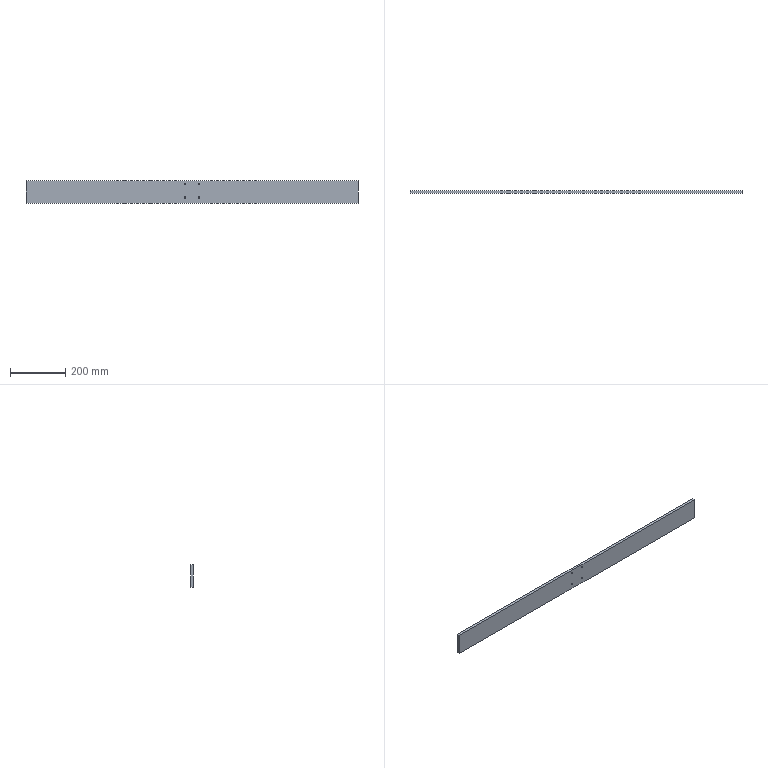Part | SolidWorks | features Extrusion 1, ICE 1 | 1 solid | 14 faces | box 1200 x 10 x 80 mm | volume 959446 mm3 | cylinder 8 | plane 6 | commonest cylinder face diameters 4.2 x8
STEP:
#1=CARTESIAN_POINT('',(-25.,-5.,-22.1));
#2=VERTEX_POINT('',#1);
#3=CARTESIAN_POINT('',(-25.,-5.,-17.9));
#4=VERTEX_POINT('',#3);
#5=CARTESIAN_POINT('',(-25.,-5.,-20.));
#6=DIRECTION('',(0.,1.,0.));
#7=DIRECTION('',(0.,0.,1.));
#8=AXIS2_PLACEMENT_3D('',#5,#6,#7);
#9=CIRCLE('',#8,2.1);
#10=EDGE_CURVE('',#2,#4,#9,.T.);
#11=ORIENTED_EDGE('',*,*,#10,.F.);
#12=CARTESIAN_POINT('',(-25.,5.,-22.1));
#13=VERTEX_POINT('',#12);
#14=CARTESIAN_POINT('',(-25.,-21.,-22.1));
#15=DIRECTION('',(0.,1.,0.));
#16=VECTOR('',#15,1000.);
#17=LINE('',#14,#16);
#18=EDGE_CURVE('',#2,#13,#17,.T.);
#19=ORIENTED_EDGE('',*,*,#18,.T.);
#20=CARTESIAN_POINT('',(-25.,5.,-17.9));
#21=VERTEX_POINT('',#20);
#22=CARTESIAN_POINT('',(-25.,5.,-20.));
#23=DIRECTION('',(0.,1.,0.));
#24=DIRECTION('',(0.,0.,1.));
#25=AXIS2_PLACEMENT_3D('',#22,#23,#24);
#26=CIRCLE('',#25,2.1);
#27=EDGE_CURVE('',#13,#21,#26,.T.);
#28=ORIENTED_EDGE('',*,*,#27,.T.);
#29=CARTESIAN_POINT('',(-25.,-21.,-17.9));
#30=DIRECTION('',(0.,1.,0.));
#31=VECTOR('',#30,1000.);
#32=LINE('',#29,#31);
#33=EDGE_CURVE('',#4,#21,#32,.T.);
#34=ORIENTED_EDGE('',*,*,#33,.F.);
#35=EDGE_LOOP('',(#11,#19,#28,#34));
#36=FACE_OUTER_BOUND('',#35,.T.);
#37=CARTESIAN_POINT('',(-25.,-21.,-20.));
#38=DIRECTION('',(0.,1.,0.));
#39=DIRECTION('',(0.,0.,1.));
#40=AXIS2_PLACEMENT_3D('',#37,#38,#39);
#41=CYLINDRICAL_SURFACE('',#40,2.1);
#42=ADVANCED_FACE('',(#36),#41,.F.);
#43=CARTESIAN_POINT('',(25.,-5.,27.9));
#44=VERTEX_POINT('',#43);
#45=CARTESIAN_POINT('',(25.,-5.,32.1));
#46=VERTEX_POINT('',#45);
#47=CARTESIAN_POINT('',(25.,-5.,30.));
#48=DIRECTION('',(0.,1.,0.));
#49=DIRECTION('',(0.,0.,1.));
#50=AXIS2_PLACEMENT_3D('',#47,#48,#49);
#51=CIRCLE('',#50,2.1);
#52=EDGE_CURVE('',#44,#46,#51,.T.);
#53=ORIENTED_EDGE('',*,*,#52,.F.);
#54=CARTESIAN_POINT('',(25.,5.,27.9));
#55=VERTEX_POINT('',#54);
#56=CARTESIAN_POINT('',(25.,-21.,27.9));
#57=DIRECTION('',(0.,1.,0.));
#58=VECTOR('',#57,1000.);
#59=LINE('',#56,#58);
#60=EDGE_CURVE('',#44,#55,#59,.T.);
#61=ORIENTED_EDGE('',*,*,#60,.T.);
#62=CARTESIAN_POINT('',(25.,5.,32.1));
#63=VERTEX_POINT('',#62);
#64=CARTESIAN_POINT('',(25.,5.,30.));
#65=DIRECTION('',(0.,1.,0.));
#66=DIRECTION('',(0.,0.,1.));
#67=AXIS2_PLACEMENT_3D('',#64,#65,#66);
#68=CIRCLE('',#67,2.1);
#69=EDGE_CURVE('',#55,#63,#68,.T.);
#70=ORIENTED_EDGE('',*,*,#69,.T.);
#71=CARTESIAN_POINT('',(25.,-21.,32.1));
#72=DIRECTION('',(0.,1.,0.));
#73=VECTOR('',#72,1000.);
#74=LINE('',#71,#73);
#75=EDGE_CURVE('',#46,#63,#74,.T.);
#76=ORIENTED_EDGE('',*,*,#75,.F.);
#77=EDGE_LOOP('',(#53,#61,#70,#76));
#78=FACE_OUTER_BOUND('',#77,.T.);
#79=CARTESIAN_POINT('',(25.,-21.,30.));
#80=DIRECTION('',(0.,1.,0.));
#81=DIRECTION('',(0.,0.,1.));
#82=AXIS2_PLACEMENT_3D('',#79,#80,#81);
#83=CYLINDRICAL_SURFACE('',#82,2.1);
#84=ADVANCED_FACE('',(#78),#83,.F.);
#85=CARTESIAN_POINT('',(-25.,-5.,27.9));
#86=VERTEX_POINT('',#85);
#87=CARTESIAN_POINT('',(-25.,-5.,32.1));
#88=VERTEX_POINT('',#87);
#89=CARTESIAN_POINT('',(-25.,-5.,30.));
#90=DIRECTION('',(0.,1.,0.));
#91=DIRECTION('',(0.,0.,1.));
#92=AXIS2_PLACEMENT_3D('',#89,#90,#91);
#93=CIRCLE('',#92,2.1);
#94=EDGE_CURVE('',#86,#88,#93,.T.);
#95=ORIENTED_EDGE('',*,*,#94,.F.);
#96=CARTESIAN_POINT('',(-25.,5.,27.9));
#97=VERTEX_POINT('',#96);
#98=CARTESIAN_POINT('',(-25.,-21.,27.9));
#99=DIRECTION('',(0.,1.,0.));
#100=VECTOR('',#99,1000.);
#101=LINE('',#98,#100);
#102=EDGE_CURVE('',#86,#97,#101,.T.);
#103=ORIENTED_EDGE('',*,*,#102,.T.);
#104=CARTESIAN_POINT('',(-25.,5.,32.1));
#105=VERTEX_POINT('',#104);
#106=CARTESIAN_POINT('',(-25.,5.,30.));
#107=DIRECTION('',(0.,1.,0.));
#108=DIRECTION('',(0.,0.,1.));
#109=AXIS2_PLACEMENT_3D('',#106,#107,#108);
#110=CIRCLE('',#109,2.1);
#111=EDGE_CURVE('',#97,#105,#110,.T.);
#112=ORIENTED_EDGE('',*,*,#111,.T.);
#113=CARTESIAN_POINT('',(-25.,-21.,32.1));
#114=DIRECTION('',(0.,1.,0.));
#115=VECTOR('',#114,1000.);
#116=LINE('',#113,#115);
#117=EDGE_CURVE('',#88,#105,#116,.T.);
#118=ORIENTED_EDGE('',*,*,#117,.F.);
#119=EDGE_LOOP('',(#95,#103,#112,#118));
#120=FACE_OUTER_BOUND('',#119,.T.);
#121=CARTESIAN_POINT('',(-25.,-21.,30.));
#122=DIRECTION('',(0.,1.,0.));
#123=DIRECTION('',(0.,0.,1.));
#124=AXIS2_PLACEMENT_3D('',#121,#122,#123);
#125=CYLINDRICAL_SURFACE('',#124,2.1);
#126=ADVANCED_FACE('',(#120),#125,.F.);
#127=CARTESIAN_POINT('',(25.,-5.,-22.1));
#128=VERTEX_POINT('',#127);
#129=CARTESIAN_POINT('',(25.,-5.,-17.9));
#130=VERTEX_POINT('',#129);
#131=CARTESIAN_POINT('',(25.,-5.,-20.));
#132=DIRECTION('',(0.,1.,0.));
#133=DIRECTION('',(0.,0.,1.));
#134=AXIS2_PLACEMENT_3D('',#131,#132,#133);
#135=CIRCLE('',#134,2.1);
#136=EDGE_CURVE('',#128,#130,#135,.T.);
#137=ORIENTED_EDGE('',*,*,#136,.F.);
#138=CARTESIAN_POINT('',(25.,5.,-22.1));
#139=VERTEX_POINT('',#138);
#140=CARTESIAN_POINT('',(25.,-21.,-22.1));
#141=DIRECTION('',(0.,1.,0.));
#142=VECTOR('',#141,1000.);
#143=LINE('',#140,#142);
#144=EDGE_CURVE('',#128,#139,#143,.T.);
#145=ORIENTED_EDGE('',*,*,#144,.T.);
#146=CARTESIAN_POINT('',(25.,5.,-17.9));
#147=VERTEX_POINT('',#146);
#148=CARTESIAN_POINT('',(25.,5.,-20.));
#149=DIRECTION('',(0.,1.,0.));
#150=DIRECTION('',(0.,0.,1.));
#151=AXIS2_PLACEMENT_3D('',#148,#149,#150);
#152=CIRCLE('',#151,2.1);
#153=EDGE_CURVE('',#139,#147,#152,.T.);
#154=ORIENTED_EDGE('',*,*,#153,.T.);
#155=CARTESIAN_POINT('',(25.,-21.,-17.9));
#156=DIRECTION('',(0.,1.,0.));
#157=VECTOR('',#156,1000.);
#158=LINE('',#155,#157);
#159=EDGE_CURVE('',#130,#147,#158,.T.);
#160=ORIENTED_EDGE('',*,*,#159,.F.);
#161=EDGE_LOOP('',(#137,#145,#154,#160));
#162=FACE_OUTER_BOUND('',#161,.T.);
#163=CARTESIAN_POINT('',(25.,-21.,-20.));
#164=DIRECTION('',(0.,1.,0.));
#165=DIRECTION('',(0.,0.,1.));
#166=AXIS2_PLACEMENT_3D('',#163,#164,#165);
#167=CYLINDRICAL_SURFACE('',#166,2.1);
#168=ADVANCED_FACE('',(#162),#167,.F.);
#169=CARTESIAN_POINT('',(600.,-5.,40.));
#170=VERTEX_POINT('',#169);
#171=CARTESIAN_POINT('',(600.,-5.,-40.));
#172=VERTEX_POINT('',#171);
#173=CARTESIAN_POINT('',(600.,-5.,-40.));
#174=DIRECTION('',(0.,0.,-1.));
#175=VECTOR('',#174,1000.);
#176=LINE('',#173,#175);
#177=EDGE_CURVE('',#170,#172,#176,.T.);
#178=ORIENTED_EDGE('',*,*,#177,.T.);
#179=CARTESIAN_POINT('',(600.,5.,-40.));
#180=VERTEX_POINT('',#179);
#181=CARTESIAN_POINT('',(600.,5.,-40.));
#182=DIRECTION('',(0.,-1.,0.));
#183=VECTOR('',#182,1000.);
#184=LINE('',#181,#183);
#185=EDGE_CURVE('',#180,#172,#184,.T.);
#186=ORIENTED_EDGE('',*,*,#185,.F.);
#187=CARTESIAN_POINT('',(600.,5.,40.));
#188=VERTEX_POINT('',#187);
#189=CARTESIAN_POINT('',(600.,5.,-40.));
#190=DIRECTION('',(0.,0.,-1.));
#191=VECTOR('',#190,1000.);
#192=LINE('',#189,#191);
#193=EDGE_CURVE('',#188,#180,#192,.T.);
#194=ORIENTED_EDGE('',*,*,#193,.F.);
#195=CARTESIAN_POINT('',(600.,5.,40.));
#196=DIRECTION('',(0.,-1.,0.));
#197=VECTOR('',#196,1000.);
#198=LINE('',#195,#197);
#199=EDGE_CURVE('',#188,#170,#198,.T.);
#200=ORIENTED_EDGE('',*,*,#199,.T.);
#201=EDGE_LOOP('',(#178,#186,#194,#200));
#202=FACE_OUTER_BOUND('',#201,.T.);
#203=CARTESIAN_POINT('',(600.,5.,-40.));
#204=DIRECTION('',(-1.,0.,0.));
#205=DIRECTION('',(0.,0.,1.));
#206=AXIS2_PLACEMENT_3D('',#203,#204,#205);
#207=PLANE('',#206);
#208=ADVANCED_FACE('',(#202),#207,.F.);
#209=CARTESIAN_POINT('',(-600.,-5.,-40.));
#210=VERTEX_POINT('',#209);
#211=CARTESIAN_POINT('',(-600.,-5.,-40.));
#212=DIRECTION('',(-1.,0.,0.));
#213=VECTOR('',#212,1000.);
#214=LINE('',#211,#213);
#215=EDGE_CURVE('',#172,#210,#214,.T.);
#216=ORIENTED_EDGE('',*,*,#215,.T.);
#217=CARTESIAN_POINT('',(-600.,5.,-40.));
#218=VERTEX_POINT('',#217);
#219=CARTESIAN_POINT('',(-600.,5.,-40.));
#220=DIRECTION('',(0.,-1.,0.));
#221=VECTOR('',#220,1000.);
#222=LINE('',#219,#221);
#223=EDGE_CURVE('',#218,#210,#222,.T.);
#224=ORIENTED_EDGE('',*,*,#223,.F.);
#225=CARTESIAN_POINT('',(-600.,5.,-40.));
#226=DIRECTION('',(-1.,0.,0.));
#227=VECTOR('',#226,1000.);
#228=LINE('',#225,#227);
#229=EDGE_CURVE('',#180,#218,#228,.T.);
#230=ORIENTED_EDGE('',*,*,#229,.F.);
#231=ORIENTED_EDGE('',*,*,#185,.T.);
#232=EDGE_LOOP('',(#216,#224,#230,#231));
#233=FACE_OUTER_BOUND('',#232,.T.);
#234=CARTESIAN_POINT('',(-600.,5.,-40.));
#235=DIRECTION('',(0.,0.,1.));
#236=DIRECTION('',(1.,0.,0.));
#237=AXIS2_PLACEMENT_3D('',#234,#235,#236);
#238=PLANE('',#237);
#239=ADVANCED_FACE('',(#233),#238,.F.);
#240=CARTESIAN_POINT('',(-600.,-5.,40.));
#241=VERTEX_POINT('',#240);
#242=CARTESIAN_POINT('',(-600.,-5.,-40.));
#243=DIRECTION('',(0.,0.,1.));
#244=VECTOR('',#243,1000.);
#245=LINE('',#242,#244);
#246=EDGE_CURVE('',#210,#241,#245,.T.);
#247=ORIENTED_EDGE('',*,*,#246,.T.);
#248=CARTESIAN_POINT('',(-600.,5.,40.));
#249=VERTEX_POINT('',#248);
#250=CARTESIAN_POINT('',(-600.,5.,40.));
#251=DIRECTION('',(0.,-1.,0.));
#252=VECTOR('',#251,1000.);
#253=LINE('',#250,#252);
#254=EDGE_CURVE('',#249,#241,#253,.T.);
#255=ORIENTED_EDGE('',*,*,#254,.F.);
#256=CARTESIAN_POINT('',(-600.,5.,-40.));
#257=DIRECTION('',(0.,0.,1.));
#258=VECTOR('',#257,1000.);
#259=LINE('',#256,#258);
#260=EDGE_CURVE('',#218,#249,#259,.T.);
#261=ORIENTED_EDGE('',*,*,#260,.F.);
#262=ORIENTED_EDGE('',*,*,#223,.T.);
#263=EDGE_LOOP('',(#247,#255,#261,#262));
#264=FACE_OUTER_BOUND('',#263,.T.);
#265=CARTESIAN_POINT('',(-600.,5.,-40.));
#266=DIRECTION('',(1.,0.,0.));
#267=DIRECTION('',(0.,0.,-1.));
#268=AXIS2_PLACEMENT_3D('',#265,#266,#267);
#269=PLANE('',#268);
#270=ADVANCED_FACE('',(#264),#269,.F.);
#271=CARTESIAN_POINT('',(-600.,-5.,40.));
#272=DIRECTION('',(1.,0.,0.));
#273=VECTOR('',#272,1000.);
#274=LINE('',#271,#273);
#275=EDGE_CURVE('',#241,#170,#274,.T.);
#276=ORIENTED_EDGE('',*,*,#275,.T.);
#277=ORIENTED_EDGE('',*,*,#199,.F.);
#278=CARTESIAN_POINT('',(-600.,5.,40.));
#279=DIRECTION('',(1.,0.,0.));
#280=VECTOR('',#279,1000.);
#281=LINE('',#278,#280);
#282=EDGE_CURVE('',#249,#188,#281,.T.);
#283=ORIENTED_EDGE('',*,*,#282,.F.);
#284=ORIENTED_EDGE('',*,*,#254,.T.);
#285=EDGE_LOOP('',(#276,#277,#283,#284));
#286=FACE_OUTER_BOUND('',#285,.T.);
#287=CARTESIAN_POINT('',(-600.,5.,40.));
#288=DIRECTION('',(0.,0.,-1.));
#289=DIRECTION('',(-1.,0.,0.));
#290=AXIS2_PLACEMENT_3D('',#287,#288,#289);
#291=PLANE('',#290);
#292=ADVANCED_FACE('',(#286),#291,.F.);
#293=CARTESIAN_POINT('',(-25.,5.,-20.));
#294=DIRECTION('',(0.,1.,0.));
#295=DIRECTION('',(0.,0.,1.));
#296=AXIS2_PLACEMENT_3D('',#293,#294,#295);
#297=CIRCLE('',#296,2.1);
#298=EDGE_CURVE('',#21,#13,#297,.T.);
#299=ORIENTED_EDGE('',*,*,#298,.F.);
#300=ORIENTED_EDGE('',*,*,#27,.F.);
#301=EDGE_LOOP('',(#299,#300));
#302=FACE_BOUND('',#301,.T.);
#303=CARTESIAN_POINT('',(25.,5.,30.));
#304=DIRECTION('',(0.,1.,0.));
#305=DIRECTION('',(0.,0.,1.));
#306=AXIS2_PLACEMENT_3D('',#303,#304,#305);
#307=CIRCLE('',#306,2.1);
#308=EDGE_CURVE('',#63,#55,#307,.T.);
#309=ORIENTED_EDGE('',*,*,#308,.F.);
#310=ORIENTED_EDGE('',*,*,#69,.F.);
#311=EDGE_LOOP('',(#309,#310));
#312=FACE_BOUND('',#311,.T.);
#313=CARTESIAN_POINT('',(-25.,5.,30.));
#314=DIRECTION('',(0.,1.,0.));
#315=DIRECTION('',(0.,0.,1.));
#316=AXIS2_PLACEMENT_3D('',#313,#314,#315);
#317=CIRCLE('',#316,2.1);
#318=EDGE_CURVE('',#105,#97,#317,.T.);
#319=ORIENTED_EDGE('',*,*,#318,.F.);
#320=ORIENTED_EDGE('',*,*,#111,.F.);
#321=EDGE_LOOP('',(#319,#320));
#322=FACE_BOUND('',#321,.T.);
#323=CARTESIAN_POINT('',(25.,5.,-20.));
#324=DIRECTION('',(0.,1.,0.));
#325=DIRECTION('',(0.,0.,1.));
#326=AXIS2_PLACEMENT_3D('',#323,#324,#325);
#327=CIRCLE('',#326,2.1);
#328=EDGE_CURVE('',#147,#139,#327,.T.);
#329=ORIENTED_EDGE('',*,*,#328,.F.);
#330=ORIENTED_EDGE('',*,*,#153,.F.);
#331=EDGE_LOOP('',(#329,#330));
#332=FACE_BOUND('',#331,.T.);
#333=ORIENTED_EDGE('',*,*,#193,.T.);
#334=ORIENTED_EDGE('',*,*,#229,.T.);
#335=ORIENTED_EDGE('',*,*,#260,.T.);
#336=ORIENTED_EDGE('',*,*,#282,.T.);
#337=EDGE_LOOP('',(#333,#334,#335,#336));
#338=FACE_OUTER_BOUND('',#337,.T.);
#339=CARTESIAN_POINT('',(0.,5.,0.));
#340=DIRECTION('',(0.,1.,0.));
#341=DIRECTION('',(0.,0.,1.));
#342=AXIS2_PLACEMENT_3D('',#339,#340,#341);
#343=PLANE('',#342);
#344=ADVANCED_FACE('',(#302,#312,#322,#332,#338),#343,.T.);
#345=CARTESIAN_POINT('',(-25.,-5.,-20.));
#346=DIRECTION('',(0.,1.,0.));
#347=DIRECTION('',(0.,0.,1.));
#348=AXIS2_PLACEMENT_3D('',#345,#346,#347);
#349=CIRCLE('',#348,2.1);
#350=EDGE_CURVE('',#4,#2,#349,.T.);
#351=ORIENTED_EDGE('',*,*,#350,.T.);
#352=ORIENTED_EDGE('',*,*,#10,.T.);
#353=EDGE_LOOP('',(#351,#352));
#354=FACE_BOUND('',#353,.T.);
#355=CARTESIAN_POINT('',(25.,-5.,30.));
#356=DIRECTION('',(0.,1.,0.));
#357=DIRECTION('',(0.,0.,1.));
#358=AXIS2_PLACEMENT_3D('',#355,#356,#357);
#359=CIRCLE('',#358,2.1);
#360=EDGE_CURVE('',#46,#44,#359,.T.);
#361=ORIENTED_EDGE('',*,*,#360,.T.);
#362=ORIENTED_EDGE('',*,*,#52,.T.);
#363=EDGE_LOOP('',(#361,#362));
#364=FACE_BOUND('',#363,.T.);
#365=CARTESIAN_POINT('',(-25.,-5.,30.));
#366=DIRECTION('',(0.,1.,0.));
#367=DIRECTION('',(0.,0.,1.));
#368=AXIS2_PLACEMENT_3D('',#365,#366,#367);
#369=CIRCLE('',#368,2.1);
#370=EDGE_CURVE('',#88,#86,#369,.T.);
#371=ORIENTED_EDGE('',*,*,#370,.T.);
#372=ORIENTED_EDGE('',*,*,#94,.T.);
#373=EDGE_LOOP('',(#371,#372));
#374=FACE_BOUND('',#373,.T.);
#375=CARTESIAN_POINT('',(25.,-5.,-20.));
#376=DIRECTION('',(0.,1.,0.));
#377=DIRECTION('',(0.,0.,1.));
#378=AXIS2_PLACEMENT_3D('',#375,#376,#377);
#379=CIRCLE('',#378,2.1);
#380=EDGE_CURVE('',#130,#128,#379,.T.);
#381=ORIENTED_EDGE('',*,*,#380,.T.);
#382=ORIENTED_EDGE('',*,*,#136,.T.);
#383=EDGE_LOOP('',(#381,#382));
#384=FACE_BOUND('',#383,.T.);
#385=ORIENTED_EDGE('',*,*,#177,.F.);
#386=ORIENTED_EDGE('',*,*,#275,.F.);
#387=ORIENTED_EDGE('',*,*,#246,.F.);
#388=ORIENTED_EDGE('',*,*,#215,.F.);
#389=EDGE_LOOP('',(#385,#386,#387,#388));
#390=FACE_OUTER_BOUND('',#389,.T.);
#391=CARTESIAN_POINT('',(0.,-5.,0.));
#392=DIRECTION('',(0.,1.,0.));
#393=DIRECTION('',(0.,0.,1.));
#394=AXIS2_PLACEMENT_3D('',#391,#392,#393);
#395=PLANE('',#394);
#396=ADVANCED_FACE('',(#354,#364,#374,#384,#390),#395,.F.);
#397=ORIENTED_EDGE('',*,*,#144,.F.);
#398=ORIENTED_EDGE('',*,*,#380,.F.);
#399=ORIENTED_EDGE('',*,*,#159,.T.);
#400=ORIENTED_EDGE('',*,*,#328,.T.);
#401=EDGE_LOOP('',(#397,#398,#399,#400));
#402=FACE_OUTER_BOUND('',#401,.T.);
#403=CARTESIAN_POINT('',(25.,-21.,-20.));
#404=DIRECTION('',(0.,1.,0.));
#405=DIRECTION('',(0.,0.,1.));
#406=AXIS2_PLACEMENT_3D('',#403,#404,#405);
#407=CYLINDRICAL_SURFACE('',#406,2.1);
#408=ADVANCED_FACE('',(#402),#407,.F.);
#409=ORIENTED_EDGE('',*,*,#102,.F.);
#410=ORIENTED_EDGE('',*,*,#370,.F.);
#411=ORIENTED_EDGE('',*,*,#117,.T.);
#412=ORIENTED_EDGE('',*,*,#318,.T.);
#413=EDGE_LOOP('',(#409,#410,#411,#412));
#414=FACE_OUTER_BOUND('',#413,.T.);
#415=CARTESIAN_POINT('',(-25.,-21.,30.));
#416=DIRECTION('',(0.,1.,0.));
#417=DIRECTION('',(0.,0.,1.));
#418=AXIS2_PLACEMENT_3D('',#415,#416,#417);
#419=CYLINDRICAL_SURFACE('',#418,2.1);
#420=ADVANCED_FACE('',(#414),#419,.F.);
#421=ORIENTED_EDGE('',*,*,#60,.F.);
#422=ORIENTED_EDGE('',*,*,#360,.F.);
#423=ORIENTED_EDGE('',*,*,#75,.T.);
#424=ORIENTED_EDGE('',*,*,#308,.T.);
#425=EDGE_LOOP('',(#421,#422,#423,#424));
#426=FACE_OUTER_BOUND('',#425,.T.);
#427=CARTESIAN_POINT('',(25.,-21.,30.));
#428=DIRECTION('',(0.,1.,0.));
#429=DIRECTION('',(0.,0.,1.));
#430=AXIS2_PLACEMENT_3D('',#427,#428,#429);
#431=CYLINDRICAL_SURFACE('',#430,2.1);
#432=ADVANCED_FACE('',(#426),#431,.F.);
#433=ORIENTED_EDGE('',*,*,#18,.F.);
#434=ORIENTED_EDGE('',*,*,#350,.F.);
#435=ORIENTED_EDGE('',*,*,#33,.T.);
#436=ORIENTED_EDGE('',*,*,#298,.T.);
#437=EDGE_LOOP('',(#433,#434,#435,#436));
#438=FACE_OUTER_BOUND('',#437,.T.);
#439=CARTESIAN_POINT('',(-25.,-21.,-20.));
#440=DIRECTION('',(0.,1.,0.));
#441=DIRECTION('',(0.,0.,1.));
#442=AXIS2_PLACEMENT_3D('',#439,#440,#441);
#443=CYLINDRICAL_SURFACE('',#442,2.1);
#444=ADVANCED_FACE('',(#438),#443,.F.);
#445=CLOSED_SHELL('',(#42,#84,#126,#168,#208,#239,#270,#292,#344,#396,#408,#420,#432,#444));
#446=MANIFOLD_SOLID_BREP('',#445);
#447=CARTESIAN_POINT('',(0.,0.,0.));
#448=DIRECTION('',(0.,0.,1.));
#449=DIRECTION('',(1.,0.,0.));
#450=AXIS2_PLACEMENT_3D('',#447,#448,#449);
#451=(LENGTH_UNIT()NAMED_UNIT(*)SI_UNIT(.MILLI.,.METRE.));
#452=UNCERTAINTY_MEASURE_WITH_UNIT(LENGTH_MEASURE(0.00001),#451,'','');
#453=(NAMED_UNIT(*)PLANE_ANGLE_UNIT()SI_UNIT($,.RADIAN.));
#454=(NAMED_UNIT(*)SI_UNIT($,.STERADIAN.)SOLID_ANGLE_UNIT());
#455=(GEOMETRIC_REPRESENTATION_CONTEXT(3)GLOBAL_UNCERTAINTY_ASSIGNED_CONTEXT((#452))GLOBAL_UNIT_ASSIGNED_CONTEXT((#451,#453,#454))REPRESENTATION_CONTEXT('',''));
#456=ADVANCED_BREP_SHAPE_REPRESENTATION('',(#446,#450),#455);